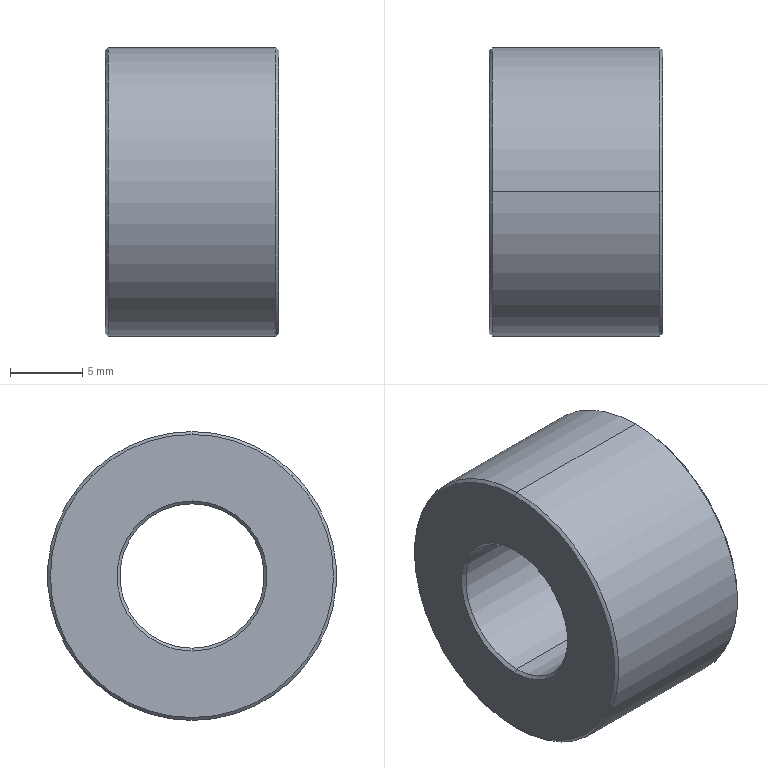Part | STEP file | NCLMH10-20-12.0 | 1 solid | 14 faces | box 12 x 20 x 20 mm | volume 2824 mm3 | cone 8 | cylinder 4 | plane 2 | commonest cylinder face diameters 10 x2 20 x2
STEP:
#1=CARTESIAN_POINT('',(12.,0.,9.8));
#2=VERTEX_POINT('',#1);
#3=CARTESIAN_POINT('',(12.,0.,-9.8));
#4=VERTEX_POINT('',#3);
#5=CARTESIAN_POINT('',(12.,0.,0.));
#6=DIRECTION('',(-1.,0.,0.));
#7=DIRECTION('',(0.,0.,1.));
#8=AXIS2_PLACEMENT_3D('',#5,#6,#7);
#9=CIRCLE('',#8,9.8);
#10=EDGE_CURVE('',#2,#4,#9,.T.);
#11=ORIENTED_EDGE('',*,*,#10,.T.);
#12=CARTESIAN_POINT('',(11.8,0.,-10.));
#13=VERTEX_POINT('',#12);
#14=CARTESIAN_POINT('',(11.8,0.,-10.));
#15=DIRECTION('',(-0.7071,0.,-0.7071));
#16=VECTOR('',#15,1000.);
#17=LINE('',#14,#16);
#18=EDGE_CURVE('',#4,#13,#17,.T.);
#19=ORIENTED_EDGE('',*,*,#18,.T.);
#20=CARTESIAN_POINT('',(11.8,0.,10.));
#21=VERTEX_POINT('',#20);
#22=CARTESIAN_POINT('',(11.8,0.,0.));
#23=DIRECTION('',(1.,0.,0.));
#24=DIRECTION('',(0.,0.,1.));
#25=AXIS2_PLACEMENT_3D('',#22,#23,#24);
#26=CIRCLE('',#25,10.);
#27=EDGE_CURVE('',#13,#21,#26,.T.);
#28=ORIENTED_EDGE('',*,*,#27,.T.);
#29=CARTESIAN_POINT('',(11.8,0.,10.));
#30=DIRECTION('',(-0.7071,0.,0.7071));
#31=VECTOR('',#30,1000.);
#32=LINE('',#29,#31);
#33=EDGE_CURVE('',#2,#21,#32,.T.);
#34=ORIENTED_EDGE('',*,*,#33,.F.);
#35=EDGE_LOOP('',(#11,#19,#28,#34));
#36=FACE_OUTER_BOUND('',#35,.T.);
#37=CARTESIAN_POINT('',(11.8,0.,0.));
#38=DIRECTION('',(-1.,0.,0.));
#39=DIRECTION('',(0.,0.,1.));
#40=AXIS2_PLACEMENT_3D('',#37,#38,#39);
#41=CONICAL_SURFACE('',#40,10.,0.7854);
#42=ADVANCED_FACE('',(#36),#41,.T.);
#43=CARTESIAN_POINT('',(11.8,0.,-5.));
#44=VERTEX_POINT('',#43);
#45=CARTESIAN_POINT('',(11.8,0.,5.));
#46=VERTEX_POINT('',#45);
#47=CARTESIAN_POINT('',(11.8,0.,0.));
#48=DIRECTION('',(-1.,0.,0.));
#49=DIRECTION('',(0.,0.,1.));
#50=AXIS2_PLACEMENT_3D('',#47,#48,#49);
#51=CIRCLE('',#50,5.);
#52=EDGE_CURVE('',#44,#46,#51,.T.);
#53=ORIENTED_EDGE('',*,*,#52,.T.);
#54=CARTESIAN_POINT('',(12.,0.,5.2));
#55=VERTEX_POINT('',#54);
#56=CARTESIAN_POINT('',(12.,0.,5.2));
#57=DIRECTION('',(0.7071,0.,0.7071));
#58=VECTOR('',#57,1000.);
#59=LINE('',#56,#58);
#60=EDGE_CURVE('',#46,#55,#59,.T.);
#61=ORIENTED_EDGE('',*,*,#60,.T.);
#62=CARTESIAN_POINT('',(12.,0.,-5.2));
#63=VERTEX_POINT('',#62);
#64=CARTESIAN_POINT('',(12.,0.,0.));
#65=DIRECTION('',(1.,0.,0.));
#66=DIRECTION('',(0.,0.,1.));
#67=AXIS2_PLACEMENT_3D('',#64,#65,#66);
#68=CIRCLE('',#67,5.2);
#69=EDGE_CURVE('',#55,#63,#68,.T.);
#70=ORIENTED_EDGE('',*,*,#69,.T.);
#71=CARTESIAN_POINT('',(12.,0.,-5.2));
#72=DIRECTION('',(0.7071,0.,-0.7071));
#73=VECTOR('',#72,1000.);
#74=LINE('',#71,#73);
#75=EDGE_CURVE('',#44,#63,#74,.T.);
#76=ORIENTED_EDGE('',*,*,#75,.F.);
#77=EDGE_LOOP('',(#53,#61,#70,#76));
#78=FACE_OUTER_BOUND('',#77,.T.);
#79=CARTESIAN_POINT('',(12.,0.,0.));
#80=DIRECTION('',(1.,0.,0.));
#81=DIRECTION('',(0.,0.,-1.));
#82=AXIS2_PLACEMENT_3D('',#79,#80,#81);
#83=CONICAL_SURFACE('',#82,5.2,0.7854);
#84=ADVANCED_FACE('',(#78),#83,.F.);
#85=CARTESIAN_POINT('',(0.,0.,-9.8));
#86=VERTEX_POINT('',#85);
#87=CARTESIAN_POINT('',(0.,0.,9.8));
#88=VERTEX_POINT('',#87);
#89=CARTESIAN_POINT('',(0.,0.,0.));
#90=DIRECTION('',(1.,0.,0.));
#91=DIRECTION('',(0.,0.,-1.));
#92=AXIS2_PLACEMENT_3D('',#89,#90,#91);
#93=CIRCLE('',#92,9.8);
#94=EDGE_CURVE('',#86,#88,#93,.T.);
#95=ORIENTED_EDGE('',*,*,#94,.T.);
#96=CARTESIAN_POINT('',(0.2,0.,10.));
#97=VERTEX_POINT('',#96);
#98=CARTESIAN_POINT('',(0.,0.,9.8));
#99=DIRECTION('',(0.7071,0.,0.7071));
#100=VECTOR('',#99,1000.);
#101=LINE('',#98,#100);
#102=EDGE_CURVE('',#88,#97,#101,.T.);
#103=ORIENTED_EDGE('',*,*,#102,.T.);
#104=CARTESIAN_POINT('',(0.2,0.,-10.));
#105=VERTEX_POINT('',#104);
#106=CARTESIAN_POINT('',(0.2,0.,0.));
#107=DIRECTION('',(-1.,0.,0.));
#108=DIRECTION('',(0.,0.,-1.));
#109=AXIS2_PLACEMENT_3D('',#106,#107,#108);
#110=CIRCLE('',#109,10.);
#111=EDGE_CURVE('',#97,#105,#110,.T.);
#112=ORIENTED_EDGE('',*,*,#111,.T.);
#113=CARTESIAN_POINT('',(0.,0.,-9.8));
#114=DIRECTION('',(0.7071,0.,-0.7071));
#115=VECTOR('',#114,1000.);
#116=LINE('',#113,#115);
#117=EDGE_CURVE('',#86,#105,#116,.T.);
#118=ORIENTED_EDGE('',*,*,#117,.F.);
#119=EDGE_LOOP('',(#95,#103,#112,#118));
#120=FACE_OUTER_BOUND('',#119,.T.);
#121=CARTESIAN_POINT('',(0.,0.,0.));
#122=DIRECTION('',(1.,0.,0.));
#123=DIRECTION('',(0.,0.,-1.));
#124=AXIS2_PLACEMENT_3D('',#121,#122,#123);
#125=CONICAL_SURFACE('',#124,9.8,0.7854);
#126=ADVANCED_FACE('',(#120),#125,.T.);
#127=CARTESIAN_POINT('',(0.2,0.,5.));
#128=VERTEX_POINT('',#127);
#129=CARTESIAN_POINT('',(0.2,0.,-5.));
#130=VERTEX_POINT('',#129);
#131=CARTESIAN_POINT('',(0.2,0.,0.));
#132=DIRECTION('',(1.,0.,0.));
#133=DIRECTION('',(0.,0.,-1.));
#134=AXIS2_PLACEMENT_3D('',#131,#132,#133);
#135=CIRCLE('',#134,5.);
#136=EDGE_CURVE('',#128,#130,#135,.T.);
#137=ORIENTED_EDGE('',*,*,#136,.T.);
#138=CARTESIAN_POINT('',(0.,0.,-5.2));
#139=VERTEX_POINT('',#138);
#140=CARTESIAN_POINT('',(0.2,0.,-5.));
#141=DIRECTION('',(-0.7071,0.,-0.7071));
#142=VECTOR('',#141,1000.);
#143=LINE('',#140,#142);
#144=EDGE_CURVE('',#130,#139,#143,.T.);
#145=ORIENTED_EDGE('',*,*,#144,.T.);
#146=CARTESIAN_POINT('',(0.,0.,5.2));
#147=VERTEX_POINT('',#146);
#148=CARTESIAN_POINT('',(0.,0.,0.));
#149=DIRECTION('',(-1.,0.,0.));
#150=DIRECTION('',(0.,0.,-1.));
#151=AXIS2_PLACEMENT_3D('',#148,#149,#150);
#152=CIRCLE('',#151,5.2);
#153=EDGE_CURVE('',#139,#147,#152,.T.);
#154=ORIENTED_EDGE('',*,*,#153,.T.);
#155=CARTESIAN_POINT('',(0.2,0.,5.));
#156=DIRECTION('',(-0.7071,0.,0.7071));
#157=VECTOR('',#156,1000.);
#158=LINE('',#155,#157);
#159=EDGE_CURVE('',#128,#147,#158,.T.);
#160=ORIENTED_EDGE('',*,*,#159,.F.);
#161=EDGE_LOOP('',(#137,#145,#154,#160));
#162=FACE_OUTER_BOUND('',#161,.T.);
#163=CARTESIAN_POINT('',(0.2,0.,0.));
#164=DIRECTION('',(-1.,0.,0.));
#165=DIRECTION('',(0.,0.,1.));
#166=AXIS2_PLACEMENT_3D('',#163,#164,#165);
#167=CONICAL_SURFACE('',#166,5.,0.7854);
#168=ADVANCED_FACE('',(#162),#167,.F.);
#169=ORIENTED_EDGE('',*,*,#52,.F.);
#170=CARTESIAN_POINT('',(0.,0.,-5.));
#171=DIRECTION('',(-1.,0.,0.));
#172=VECTOR('',#171,1000.);
#173=LINE('',#170,#172);
#174=EDGE_CURVE('',#44,#130,#173,.T.);
#175=ORIENTED_EDGE('',*,*,#174,.T.);
#176=ORIENTED_EDGE('',*,*,#136,.F.);
#177=CARTESIAN_POINT('',(0.,0.,5.));
#178=DIRECTION('',(-1.,0.,0.));
#179=VECTOR('',#178,1000.);
#180=LINE('',#177,#179);
#181=EDGE_CURVE('',#46,#128,#180,.T.);
#182=ORIENTED_EDGE('',*,*,#181,.F.);
#183=EDGE_LOOP('',(#169,#175,#176,#182));
#184=FACE_OUTER_BOUND('',#183,.T.);
#185=CARTESIAN_POINT('',(0.,0.,0.));
#186=DIRECTION('',(-1.,0.,0.));
#187=DIRECTION('',(0.,0.,1.));
#188=AXIS2_PLACEMENT_3D('',#185,#186,#187);
#189=CYLINDRICAL_SURFACE('',#188,5.);
#190=ADVANCED_FACE('',(#184),#189,.F.);
#191=ORIENTED_EDGE('',*,*,#27,.F.);
#192=CARTESIAN_POINT('',(0.,0.,-10.));
#193=DIRECTION('',(-1.,0.,0.));
#194=VECTOR('',#193,1000.);
#195=LINE('',#192,#194);
#196=EDGE_CURVE('',#13,#105,#195,.T.);
#197=ORIENTED_EDGE('',*,*,#196,.T.);
#198=ORIENTED_EDGE('',*,*,#111,.F.);
#199=CARTESIAN_POINT('',(0.,0.,10.));
#200=DIRECTION('',(-1.,0.,0.));
#201=VECTOR('',#200,1000.);
#202=LINE('',#199,#201);
#203=EDGE_CURVE('',#21,#97,#202,.T.);
#204=ORIENTED_EDGE('',*,*,#203,.F.);
#205=EDGE_LOOP('',(#191,#197,#198,#204));
#206=FACE_OUTER_BOUND('',#205,.T.);
#207=CARTESIAN_POINT('',(0.,0.,0.));
#208=DIRECTION('',(-1.,0.,0.));
#209=DIRECTION('',(0.,0.,1.));
#210=AXIS2_PLACEMENT_3D('',#207,#208,#209);
#211=CYLINDRICAL_SURFACE('',#210,10.);
#212=ADVANCED_FACE('',(#206),#211,.T.);
#213=CARTESIAN_POINT('',(0.,0.,0.));
#214=DIRECTION('',(-1.,0.,0.));
#215=DIRECTION('',(0.,0.,-1.));
#216=AXIS2_PLACEMENT_3D('',#213,#214,#215);
#217=CIRCLE('',#216,5.2);
#218=EDGE_CURVE('',#147,#139,#217,.T.);
#219=ORIENTED_EDGE('',*,*,#218,.F.);
#220=ORIENTED_EDGE('',*,*,#153,.F.);
#221=EDGE_LOOP('',(#219,#220));
#222=FACE_BOUND('',#221,.T.);
#223=ORIENTED_EDGE('',*,*,#94,.F.);
#224=CARTESIAN_POINT('',(0.,0.,0.));
#225=DIRECTION('',(1.,0.,0.));
#226=DIRECTION('',(0.,0.,-1.));
#227=AXIS2_PLACEMENT_3D('',#224,#225,#226);
#228=CIRCLE('',#227,9.8);
#229=EDGE_CURVE('',#88,#86,#228,.T.);
#230=ORIENTED_EDGE('',*,*,#229,.F.);
#231=EDGE_LOOP('',(#223,#230));
#232=FACE_OUTER_BOUND('',#231,.T.);
#233=CARTESIAN_POINT('',(0.,-5.,0.));
#234=DIRECTION('',(1.,0.,0.));
#235=DIRECTION('',(0.,0.,-1.));
#236=AXIS2_PLACEMENT_3D('',#233,#234,#235);
#237=PLANE('',#236);
#238=ADVANCED_FACE('',(#222,#232),#237,.F.);
#239=ORIENTED_EDGE('',*,*,#196,.F.);
#240=CARTESIAN_POINT('',(11.8,0.,0.));
#241=DIRECTION('',(1.,0.,0.));
#242=DIRECTION('',(0.,0.,1.));
#243=AXIS2_PLACEMENT_3D('',#240,#241,#242);
#244=CIRCLE('',#243,10.);
#245=EDGE_CURVE('',#21,#13,#244,.T.);
#246=ORIENTED_EDGE('',*,*,#245,.F.);
#247=ORIENTED_EDGE('',*,*,#203,.T.);
#248=CARTESIAN_POINT('',(0.2,0.,0.));
#249=DIRECTION('',(-1.,0.,0.));
#250=DIRECTION('',(0.,0.,-1.));
#251=AXIS2_PLACEMENT_3D('',#248,#249,#250);
#252=CIRCLE('',#251,10.);
#253=EDGE_CURVE('',#105,#97,#252,.T.);
#254=ORIENTED_EDGE('',*,*,#253,.F.);
#255=EDGE_LOOP('',(#239,#246,#247,#254));
#256=FACE_OUTER_BOUND('',#255,.T.);
#257=CARTESIAN_POINT('',(0.,0.,0.));
#258=DIRECTION('',(-1.,0.,0.));
#259=DIRECTION('',(0.,0.,1.));
#260=AXIS2_PLACEMENT_3D('',#257,#258,#259);
#261=CYLINDRICAL_SURFACE('',#260,10.);
#262=ADVANCED_FACE('',(#256),#261,.T.);
#263=CARTESIAN_POINT('',(12.,0.,0.));
#264=DIRECTION('',(1.,0.,0.));
#265=DIRECTION('',(0.,0.,1.));
#266=AXIS2_PLACEMENT_3D('',#263,#264,#265);
#267=CIRCLE('',#266,5.2);
#268=EDGE_CURVE('',#63,#55,#267,.T.);
#269=ORIENTED_EDGE('',*,*,#268,.F.);
#270=ORIENTED_EDGE('',*,*,#69,.F.);
#271=EDGE_LOOP('',(#269,#270));
#272=FACE_BOUND('',#271,.T.);
#273=ORIENTED_EDGE('',*,*,#10,.F.);
#274=CARTESIAN_POINT('',(12.,0.,0.));
#275=DIRECTION('',(-1.,0.,0.));
#276=DIRECTION('',(0.,0.,1.));
#277=AXIS2_PLACEMENT_3D('',#274,#275,#276);
#278=CIRCLE('',#277,9.8);
#279=EDGE_CURVE('',#4,#2,#278,.T.);
#280=ORIENTED_EDGE('',*,*,#279,.F.);
#281=EDGE_LOOP('',(#273,#280));
#282=FACE_OUTER_BOUND('',#281,.T.);
#283=CARTESIAN_POINT('',(12.,-5.,0.));
#284=DIRECTION('',(-1.,0.,0.));
#285=DIRECTION('',(0.,0.,1.));
#286=AXIS2_PLACEMENT_3D('',#283,#284,#285);
#287=PLANE('',#286);
#288=ADVANCED_FACE('',(#272,#282),#287,.F.);
#289=ORIENTED_EDGE('',*,*,#174,.F.);
#290=CARTESIAN_POINT('',(11.8,0.,0.));
#291=DIRECTION('',(-1.,0.,0.));
#292=DIRECTION('',(0.,0.,1.));
#293=AXIS2_PLACEMENT_3D('',#290,#291,#292);
#294=CIRCLE('',#293,5.);
#295=EDGE_CURVE('',#46,#44,#294,.T.);
#296=ORIENTED_EDGE('',*,*,#295,.F.);
#297=ORIENTED_EDGE('',*,*,#181,.T.);
#298=CARTESIAN_POINT('',(0.2,0.,0.));
#299=DIRECTION('',(1.,0.,0.));
#300=DIRECTION('',(0.,0.,-1.));
#301=AXIS2_PLACEMENT_3D('',#298,#299,#300);
#302=CIRCLE('',#301,5.);
#303=EDGE_CURVE('',#130,#128,#302,.T.);
#304=ORIENTED_EDGE('',*,*,#303,.F.);
#305=EDGE_LOOP('',(#289,#296,#297,#304));
#306=FACE_OUTER_BOUND('',#305,.T.);
#307=CARTESIAN_POINT('',(0.,0.,0.));
#308=DIRECTION('',(-1.,0.,0.));
#309=DIRECTION('',(0.,0.,1.));
#310=AXIS2_PLACEMENT_3D('',#307,#308,#309);
#311=CYLINDRICAL_SURFACE('',#310,5.);
#312=ADVANCED_FACE('',(#306),#311,.F.);
#313=ORIENTED_EDGE('',*,*,#144,.F.);
#314=ORIENTED_EDGE('',*,*,#303,.T.);
#315=ORIENTED_EDGE('',*,*,#159,.T.);
#316=ORIENTED_EDGE('',*,*,#218,.T.);
#317=EDGE_LOOP('',(#313,#314,#315,#316));
#318=FACE_OUTER_BOUND('',#317,.T.);
#319=CARTESIAN_POINT('',(0.2,0.,0.));
#320=DIRECTION('',(-1.,0.,0.));
#321=DIRECTION('',(0.,0.,1.));
#322=AXIS2_PLACEMENT_3D('',#319,#320,#321);
#323=CONICAL_SURFACE('',#322,5.,0.7854);
#324=ADVANCED_FACE('',(#318),#323,.F.);
#325=ORIENTED_EDGE('',*,*,#102,.F.);
#326=ORIENTED_EDGE('',*,*,#229,.T.);
#327=ORIENTED_EDGE('',*,*,#117,.T.);
#328=ORIENTED_EDGE('',*,*,#253,.T.);
#329=EDGE_LOOP('',(#325,#326,#327,#328));
#330=FACE_OUTER_BOUND('',#329,.T.);
#331=CARTESIAN_POINT('',(0.,0.,0.));
#332=DIRECTION('',(1.,0.,0.));
#333=DIRECTION('',(0.,0.,-1.));
#334=AXIS2_PLACEMENT_3D('',#331,#332,#333);
#335=CONICAL_SURFACE('',#334,9.8,0.7854);
#336=ADVANCED_FACE('',(#330),#335,.T.);
#337=ORIENTED_EDGE('',*,*,#60,.F.);
#338=ORIENTED_EDGE('',*,*,#295,.T.);
#339=ORIENTED_EDGE('',*,*,#75,.T.);
#340=ORIENTED_EDGE('',*,*,#268,.T.);
#341=EDGE_LOOP('',(#337,#338,#339,#340));
#342=FACE_OUTER_BOUND('',#341,.T.);
#343=CARTESIAN_POINT('',(12.,0.,0.));
#344=DIRECTION('',(1.,0.,0.));
#345=DIRECTION('',(0.,0.,-1.));
#346=AXIS2_PLACEMENT_3D('',#343,#344,#345);
#347=CONICAL_SURFACE('',#346,5.2,0.7854);
#348=ADVANCED_FACE('',(#342),#347,.F.);
#349=ORIENTED_EDGE('',*,*,#18,.F.);
#350=ORIENTED_EDGE('',*,*,#279,.T.);
#351=ORIENTED_EDGE('',*,*,#33,.T.);
#352=ORIENTED_EDGE('',*,*,#245,.T.);
#353=EDGE_LOOP('',(#349,#350,#351,#352));
#354=FACE_OUTER_BOUND('',#353,.T.);
#355=CARTESIAN_POINT('',(11.8,0.,0.));
#356=DIRECTION('',(-1.,0.,0.));
#357=DIRECTION('',(0.,0.,1.));
#358=AXIS2_PLACEMENT_3D('',#355,#356,#357);
#359=CONICAL_SURFACE('',#358,10.,0.7854);
#360=ADVANCED_FACE('',(#354),#359,.T.);
#361=CLOSED_SHELL('',(#42,#84,#126,#168,#190,#212,#238,#262,#288,#312,#324,#336,#348,#360));
#362=MANIFOLD_SOLID_BREP('',#361);
#363=CARTESIAN_POINT('',(0.,0.,0.));
#364=DIRECTION('',(0.,0.,1.));
#365=DIRECTION('',(1.,0.,0.));
#366=AXIS2_PLACEMENT_3D('',#363,#364,#365);
#367=(LENGTH_UNIT()NAMED_UNIT(*)SI_UNIT(.MILLI.,.METRE.));
#368=UNCERTAINTY_MEASURE_WITH_UNIT(LENGTH_MEASURE(0.00001),#367,'','');
#369=(NAMED_UNIT(*)PLANE_ANGLE_UNIT()SI_UNIT($,.RADIAN.));
#370=(NAMED_UNIT(*)SI_UNIT($,.STERADIAN.)SOLID_ANGLE_UNIT());
#371=(GEOMETRIC_REPRESENTATION_CONTEXT(3)GLOBAL_UNCERTAINTY_ASSIGNED_CONTEXT((#368))GLOBAL_UNIT_ASSIGNED_CONTEXT((#367,#369,#370))REPRESENTATION_CONTEXT('',''));
#372=ADVANCED_BREP_SHAPE_REPRESENTATION('',(#362,#366),#371);